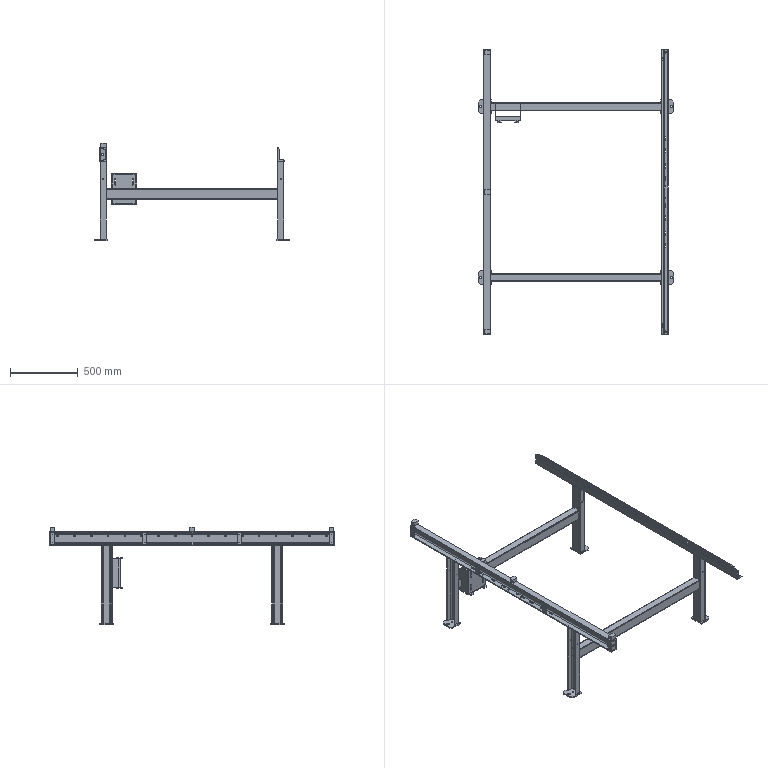Part | SolidWorks | features CompositeCurve 2 | 26 solids | 789 faces | box 1444 x 2100 x 717 mm | volume 11597718 mm3 | plane 400 | cylinder 389 | commonest cylinder face diameters 13 x76 6 x68 10.5 x48 5 x40 20 x38 11 x36